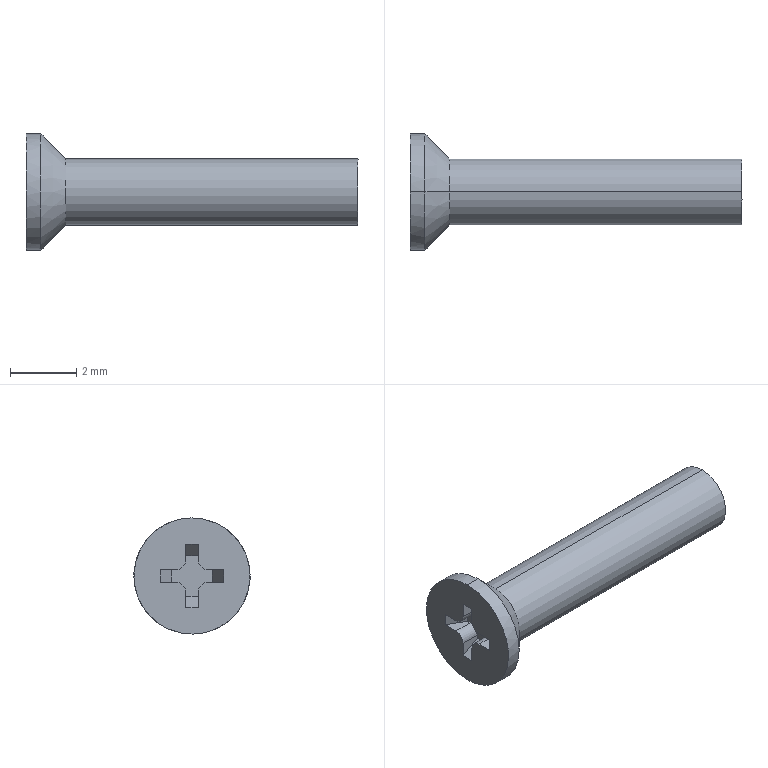Part | STEP file | PN_0016_Default<As Machined> | 1 solid | 25 faces | box 10 x 3.5 x 3.5 mm | volume 35.87 mm3 | plane 15 | cylinder 8 | cone 2 | commonest cylinder face diameters 0.6 x4 2 x2 3.5 x2
STEP:
#1=CARTESIAN_POINT('',(1.2,0.,-1.));
#2=VERTEX_POINT('',#1);
#3=CARTESIAN_POINT('',(1.2,0.,1.));
#4=VERTEX_POINT('',#3);
#5=CARTESIAN_POINT('',(1.2,0.,0.));
#6=DIRECTION('',(1.,0.,0.));
#7=AXIS2_PLACEMENT_3D('',#5,#6,$);
#8=CIRCLE('',#7,1.);
#9=EDGE_CURVE('',#2,#4,#8,.T.);
#10=ORIENTED_EDGE('',*,*,#9,.T.);
#11=CARTESIAN_POINT('',(10.,0.,1.));
#12=VERTEX_POINT('',#11);
#13=CARTESIAN_POINT('',(4.516,0.,1.));
#14=DIRECTION('',(1.,0.,0.));
#15=VECTOR('',#14,1.);
#16=LINE('',#13,#15);
#17=EDGE_CURVE('',#4,#12,#16,.T.);
#18=ORIENTED_EDGE('',*,*,#17,.T.);
#19=CARTESIAN_POINT('',(10.,0.,-1.));
#20=VERTEX_POINT('',#19);
#21=CARTESIAN_POINT('',(10.,0.,0.));
#22=DIRECTION('',(1.,0.,0.));
#23=AXIS2_PLACEMENT_3D('',#21,#22,$);
#24=CIRCLE('',#23,1.);
#25=EDGE_CURVE('',#20,#12,#24,.T.);
#26=ORIENTED_EDGE('',*,*,#25,.F.);
#27=CARTESIAN_POINT('',(4.516,0.,-1.));
#28=DIRECTION('',(1.,0.,0.));
#29=VECTOR('',#28,1.);
#30=LINE('',#27,#29);
#31=EDGE_CURVE('',#2,#20,#30,.T.);
#32=ORIENTED_EDGE('',*,*,#31,.F.);
#33=EDGE_LOOP('',(#10,#18,#26,#32));
#34=FACE_OUTER_BOUND('',#33,.T.);
#35=CARTESIAN_POINT('',(4.516,0.,0.));
#36=DIRECTION('',(1.,0.,0.));
#37=DIRECTION('',(0.,0.,-1.));
#38=AXIS2_PLACEMENT_3D('',#35,#36,#37);
#39=CYLINDRICAL_SURFACE('',#38,1.);
#40=ADVANCED_FACE('',(#34),#39,.T.);
#41=ORIENTED_EDGE('',*,*,#9,.F.);
#42=CARTESIAN_POINT('',(0.45,0.,-1.75));
#43=VERTEX_POINT('',#42);
#44=CARTESIAN_POINT('',(-353551.691,0.,-353553.891));
#45=DIRECTION('',(-0.7071,0.,-0.7071));
#46=VECTOR('',#45,1.);
#47=LINE('',#44,#46);
#48=EDGE_CURVE('',#2,#43,#47,.T.);
#49=ORIENTED_EDGE('',*,*,#48,.T.);
#50=CARTESIAN_POINT('',(0.45,0.,1.75));
#51=VERTEX_POINT('',#50);
#52=CARTESIAN_POINT('',(0.45,0.,0.));
#53=DIRECTION('',(-1.,0.,0.));
#54=AXIS2_PLACEMENT_3D('',#52,#53,$);
#55=CIRCLE('',#54,1.75);
#56=EDGE_CURVE('',#43,#51,#55,.F.);
#57=ORIENTED_EDGE('',*,*,#56,.T.);
#58=CARTESIAN_POINT('',(-353551.691,0.,353553.891));
#59=DIRECTION('',(-0.7071,0.,0.7071));
#60=VECTOR('',#59,1.);
#61=LINE('',#58,#60);
#62=EDGE_CURVE('',#4,#51,#61,.T.);
#63=ORIENTED_EDGE('',*,*,#62,.F.);
#64=EDGE_LOOP('',(#41,#49,#57,#63));
#65=FACE_OUTER_BOUND('',#64,.T.);
#66=CARTESIAN_POINT('',(1.2,0.,0.));
#67=DIRECTION('',(-1.,0.,0.));
#68=DIRECTION('',(0.,0.,1.));
#69=AXIS2_PLACEMENT_3D('',#66,#67,#68);
#70=CONICAL_SURFACE('',#69,1.,0.7854);
#71=ADVANCED_FACE('',(#65),#70,.T.);
#72=ORIENTED_EDGE('',*,*,#17,.F.);
#73=CARTESIAN_POINT('',(1.2,0.,1.));
#74=CARTESIAN_POINT('',(1.2,-0.3142,1.));
#75=CARTESIAN_POINT('',(1.2,-0.6283,0.8766));
#76=CARTESIAN_POINT('',(1.2,-0.8766,0.6283));
#77=CARTESIAN_POINT('',(1.2,-1.123,0.));
#78=CARTESIAN_POINT('',(1.2,-0.8766,-0.6283));
#79=CARTESIAN_POINT('',(1.2,-0.6283,-0.8766));
#80=CARTESIAN_POINT('',(1.2,-0.3142,-1.));
#81=CARTESIAN_POINT('',(1.2,0.,-1.));
#82=B_SPLINE_CURVE_WITH_KNOTS('',5,(#73,#74,#75,#76,#77,#78,#79,#80,#81),.UNSPECIFIED.,.F.,.U.,(6,3,6),(-1.571,0.,1.571),.UNSPECIFIED.);
#83=EDGE_CURVE('',#4,#2,#82,.T.);
#84=ORIENTED_EDGE('',*,*,#83,.T.);
#85=ORIENTED_EDGE('',*,*,#31,.T.);
#86=CARTESIAN_POINT('',(10.,0.,1.));
#87=CARTESIAN_POINT('',(10.,-0.3142,1.));
#88=CARTESIAN_POINT('',(10.,-0.6283,0.8766));
#89=CARTESIAN_POINT('',(10.,-0.8766,0.6283));
#90=CARTESIAN_POINT('',(10.,-1.123,0.));
#91=CARTESIAN_POINT('',(10.,-0.8766,-0.6283));
#92=CARTESIAN_POINT('',(10.,-0.6283,-0.8766));
#93=CARTESIAN_POINT('',(10.,-0.3142,-1.));
#94=CARTESIAN_POINT('',(10.,0.,-1.));
#95=B_SPLINE_CURVE_WITH_KNOTS('',5,(#86,#87,#88,#89,#90,#91,#92,#93,#94),.UNSPECIFIED.,.F.,.U.,(6,3,6),(-1.571,0.,1.571),.UNSPECIFIED.);
#96=EDGE_CURVE('',#12,#20,#95,.T.);
#97=ORIENTED_EDGE('',*,*,#96,.F.);
#98=EDGE_LOOP('',(#72,#84,#85,#97));
#99=FACE_OUTER_BOUND('',#98,.T.);
#100=CARTESIAN_POINT('',(4.516,0.,0.));
#101=DIRECTION('',(1.,0.,0.));
#102=DIRECTION('',(0.,0.,1.));
#103=AXIS2_PLACEMENT_3D('',#100,#101,#102);
#104=CYLINDRICAL_SURFACE('',#103,1.);
#105=ADVANCED_FACE('',(#99),#104,.T.);
#106=ORIENTED_EDGE('',*,*,#25,.T.);
#107=ORIENTED_EDGE('',*,*,#96,.T.);
#108=EDGE_LOOP('',(#106,#107));
#109=FACE_OUTER_BOUND('',#108,.T.);
#110=CARTESIAN_POINT('',(10.,1.,0.));
#111=DIRECTION('',(1.,0.,0.));
#112=DIRECTION('',(0.,0.,-1.));
#113=AXIS2_PLACEMENT_3D('',#110,#111,#112);
#114=PLANE('',#113);
#115=ADVANCED_FACE('',(#109),#114,.T.);
#116=ORIENTED_EDGE('',*,*,#48,.F.);
#117=ORIENTED_EDGE('',*,*,#83,.F.);
#118=ORIENTED_EDGE('',*,*,#62,.T.);
#119=CARTESIAN_POINT('',(0.45,0.,0.));
#120=DIRECTION('',(-1.,0.,0.));
#121=AXIS2_PLACEMENT_3D('',#119,#120,$);
#122=CIRCLE('',#121,1.75);
#123=EDGE_CURVE('',#51,#43,#122,.F.);
#124=ORIENTED_EDGE('',*,*,#123,.T.);
#125=EDGE_LOOP('',(#116,#117,#118,#124));
#126=FACE_OUTER_BOUND('',#125,.T.);
#127=CARTESIAN_POINT('',(1.2,0.,0.));
#128=DIRECTION('',(-1.,0.,0.));
#129=DIRECTION('',(0.,0.,-1.));
#130=AXIS2_PLACEMENT_3D('',#127,#128,#129);
#131=CONICAL_SURFACE('',#130,1.,0.7854);
#132=ADVANCED_FACE('',(#126),#131,.T.);
#133=CARTESIAN_POINT('',(0.,0.,-1.75));
#134=VERTEX_POINT('',#133);
#135=CARTESIAN_POINT('',(0.,0.,1.75));
#136=VERTEX_POINT('',#135);
#137=CARTESIAN_POINT('',(0.,0.,-1.75));
#138=CARTESIAN_POINT('',(0.,0.5498,-1.75));
#139=CARTESIAN_POINT('',(0.,1.1,-1.534));
#140=CARTESIAN_POINT('',(0.,1.534,-1.1));
#141=CARTESIAN_POINT('',(0.,1.966,0.));
#142=CARTESIAN_POINT('',(0.,1.534,1.1));
#143=CARTESIAN_POINT('',(0.,1.1,1.534));
#144=CARTESIAN_POINT('',(0.,0.5498,1.75));
#145=CARTESIAN_POINT('',(0.,0.,1.75));
#146=B_SPLINE_CURVE_WITH_KNOTS('',5,(#137,#138,#139,#140,#141,#142,#143,#144,#145),.UNSPECIFIED.,.F.,.U.,(6,3,6),(-2.749,0.,2.749),.UNSPECIFIED.);
#147=EDGE_CURVE('',#134,#136,#146,.T.);
#148=ORIENTED_EDGE('',*,*,#147,.T.);
#149=CARTESIAN_POINT('',(4.516,0.,1.75));
#150=DIRECTION('',(1.,0.,0.));
#151=VECTOR('',#150,1.);
#152=LINE('',#149,#151);
#153=EDGE_CURVE('',#136,#51,#152,.T.);
#154=ORIENTED_EDGE('',*,*,#153,.T.);
#155=ORIENTED_EDGE('',*,*,#56,.F.);
#156=CARTESIAN_POINT('',(4.516,0.,-1.75));
#157=DIRECTION('',(1.,0.,0.));
#158=VECTOR('',#157,1.);
#159=LINE('',#156,#158);
#160=EDGE_CURVE('',#134,#43,#159,.T.);
#161=ORIENTED_EDGE('',*,*,#160,.F.);
#162=EDGE_LOOP('',(#148,#154,#155,#161));
#163=FACE_OUTER_BOUND('',#162,.T.);
#164=CARTESIAN_POINT('',(4.516,0.,0.));
#165=DIRECTION('',(1.,0.,0.));
#166=DIRECTION('',(0.,0.,-1.));
#167=AXIS2_PLACEMENT_3D('',#164,#165,#166);
#168=CYLINDRICAL_SURFACE('',#167,1.75);
#169=ADVANCED_FACE('',(#163),#168,.T.);
#170=ORIENTED_EDGE('',*,*,#153,.F.);
#171=CARTESIAN_POINT('',(0.,0.,1.75));
#172=CARTESIAN_POINT('',(0.,-0.5498,1.75));
#173=CARTESIAN_POINT('',(0.,-1.1,1.534));
#174=CARTESIAN_POINT('',(0.,-1.534,1.1));
#175=CARTESIAN_POINT('',(0.,-1.966,0.));
#176=CARTESIAN_POINT('',(0.,-1.534,-1.1));
#177=CARTESIAN_POINT('',(0.,-1.1,-1.534));
#178=CARTESIAN_POINT('',(0.,-0.5498,-1.75));
#179=CARTESIAN_POINT('',(0.,0.,-1.75));
#180=B_SPLINE_CURVE_WITH_KNOTS('',5,(#171,#172,#173,#174,#175,#176,#177,#178,#179),.UNSPECIFIED.,.F.,.U.,(6,3,6),(-2.749,0.,2.749),.UNSPECIFIED.);
#181=EDGE_CURVE('',#136,#134,#180,.T.);
#182=ORIENTED_EDGE('',*,*,#181,.T.);
#183=ORIENTED_EDGE('',*,*,#160,.T.);
#184=ORIENTED_EDGE('',*,*,#123,.F.);
#185=EDGE_LOOP('',(#170,#182,#183,#184));
#186=FACE_OUTER_BOUND('',#185,.T.);
#187=CARTESIAN_POINT('',(4.516,0.,0.));
#188=DIRECTION('',(1.,0.,0.));
#189=DIRECTION('',(0.,0.,1.));
#190=AXIS2_PLACEMENT_3D('',#187,#188,#189);
#191=CYLINDRICAL_SURFACE('',#190,1.75);
#192=ADVANCED_FACE('',(#186),#191,.T.);
#193=ORIENTED_EDGE('',*,*,#147,.F.);
#194=ORIENTED_EDGE('',*,*,#181,.F.);
#195=EDGE_LOOP('',(#193,#194));
#196=FACE_OUTER_BOUND('',#195,.T.);
#197=CARTESIAN_POINT('',(0.,-0.95,-0.19));
#198=VERTEX_POINT('',#197);
#199=CARTESIAN_POINT('',(0.,-0.49,-0.19));
#200=VERTEX_POINT('',#199);
#201=CARTESIAN_POINT('',(0.,-0.72,-0.19));
#202=DIRECTION('',(0.,1.,0.));
#203=VECTOR('',#202,1.);
#204=LINE('',#201,#203);
#205=EDGE_CURVE('',#198,#200,#204,.T.);
#206=ORIENTED_EDGE('',*,*,#205,.T.);
#207=CARTESIAN_POINT('',(0.,-0.19,-0.49));
#208=VERTEX_POINT('',#207);
#209=CARTESIAN_POINT('',(0.,-0.49,-0.49));
#210=DIRECTION('',(-1.,0.,0.));
#211=AXIS2_PLACEMENT_3D('',#209,#210,$);
#212=CIRCLE('',#211,0.3);
#213=EDGE_CURVE('',#200,#208,#212,.T.);
#214=ORIENTED_EDGE('',*,*,#213,.T.);
#215=CARTESIAN_POINT('',(0.,-0.19,-0.95));
#216=VERTEX_POINT('',#215);
#217=CARTESIAN_POINT('',(0.,-0.19,-0.72));
#218=DIRECTION('',(0.,0.,-1.));
#219=VECTOR('',#218,1.);
#220=LINE('',#217,#219);
#221=EDGE_CURVE('',#208,#216,#220,.T.);
#222=ORIENTED_EDGE('',*,*,#221,.T.);
#223=CARTESIAN_POINT('',(0.,0.19,-0.95));
#224=VERTEX_POINT('',#223);
#225=CARTESIAN_POINT('',(0.,0.,-0.95));
#226=DIRECTION('',(0.,1.,0.));
#227=VECTOR('',#226,1.);
#228=LINE('',#225,#227);
#229=EDGE_CURVE('',#216,#224,#228,.T.);
#230=ORIENTED_EDGE('',*,*,#229,.T.);
#231=CARTESIAN_POINT('',(0.,0.19,-0.49));
#232=VERTEX_POINT('',#231);
#233=CARTESIAN_POINT('',(0.,0.19,-0.72));
#234=DIRECTION('',(0.,0.,1.));
#235=VECTOR('',#234,1.);
#236=LINE('',#233,#235);
#237=EDGE_CURVE('',#224,#232,#236,.T.);
#238=ORIENTED_EDGE('',*,*,#237,.T.);
#239=CARTESIAN_POINT('',(0.,0.49,-0.19));
#240=VERTEX_POINT('',#239);
#241=CARTESIAN_POINT('',(0.,0.49,-0.49));
#242=DIRECTION('',(-1.,0.,0.));
#243=AXIS2_PLACEMENT_3D('',#241,#242,$);
#244=CIRCLE('',#243,0.3);
#245=EDGE_CURVE('',#232,#240,#244,.T.);
#246=ORIENTED_EDGE('',*,*,#245,.T.);
#247=CARTESIAN_POINT('',(0.,0.95,-0.19));
#248=VERTEX_POINT('',#247);
#249=CARTESIAN_POINT('',(0.,0.72,-0.19));
#250=DIRECTION('',(0.,1.,0.));
#251=VECTOR('',#250,1.);
#252=LINE('',#249,#251);
#253=EDGE_CURVE('',#240,#248,#252,.T.);
#254=ORIENTED_EDGE('',*,*,#253,.T.);
#255=CARTESIAN_POINT('',(0.,0.95,0.19));
#256=VERTEX_POINT('',#255);
#257=CARTESIAN_POINT('',(0.,0.95,0.));
#258=DIRECTION('',(0.,0.,1.));
#259=VECTOR('',#258,1.);
#260=LINE('',#257,#259);
#261=EDGE_CURVE('',#248,#256,#260,.T.);
#262=ORIENTED_EDGE('',*,*,#261,.T.);
#263=CARTESIAN_POINT('',(0.,0.49,0.19));
#264=VERTEX_POINT('',#263);
#265=CARTESIAN_POINT('',(0.,0.72,0.19));
#266=DIRECTION('',(0.,-1.,0.));
#267=VECTOR('',#266,1.);
#268=LINE('',#265,#267);
#269=EDGE_CURVE('',#256,#264,#268,.T.);
#270=ORIENTED_EDGE('',*,*,#269,.T.);
#271=CARTESIAN_POINT('',(0.,0.19,0.49));
#272=VERTEX_POINT('',#271);
#273=CARTESIAN_POINT('',(0.,0.49,0.49));
#274=DIRECTION('',(-1.,0.,0.));
#275=AXIS2_PLACEMENT_3D('',#273,#274,$);
#276=CIRCLE('',#275,0.3);
#277=EDGE_CURVE('',#264,#272,#276,.T.);
#278=ORIENTED_EDGE('',*,*,#277,.T.);
#279=CARTESIAN_POINT('',(0.,0.19,0.95));
#280=VERTEX_POINT('',#279);
#281=CARTESIAN_POINT('',(0.,0.19,0.72));
#282=DIRECTION('',(0.,0.,1.));
#283=VECTOR('',#282,1.);
#284=LINE('',#281,#283);
#285=EDGE_CURVE('',#272,#280,#284,.T.);
#286=ORIENTED_EDGE('',*,*,#285,.T.);
#287=CARTESIAN_POINT('',(0.,-0.19,0.95));
#288=VERTEX_POINT('',#287);
#289=CARTESIAN_POINT('',(0.,0.,0.95));
#290=DIRECTION('',(0.,-1.,0.));
#291=VECTOR('',#290,1.);
#292=LINE('',#289,#291);
#293=EDGE_CURVE('',#280,#288,#292,.T.);
#294=ORIENTED_EDGE('',*,*,#293,.T.);
#295=CARTESIAN_POINT('',(0.,-0.19,0.49));
#296=VERTEX_POINT('',#295);
#297=CARTESIAN_POINT('',(0.,-0.19,0.72));
#298=DIRECTION('',(0.,0.,-1.));
#299=VECTOR('',#298,1.);
#300=LINE('',#297,#299);
#301=EDGE_CURVE('',#288,#296,#300,.T.);
#302=ORIENTED_EDGE('',*,*,#301,.T.);
#303=CARTESIAN_POINT('',(0.,-0.49,0.19));
#304=VERTEX_POINT('',#303);
#305=CARTESIAN_POINT('',(0.,-0.49,0.49));
#306=DIRECTION('',(-1.,0.,0.));
#307=AXIS2_PLACEMENT_3D('',#305,#306,$);
#308=CIRCLE('',#307,0.3);
#309=EDGE_CURVE('',#296,#304,#308,.T.);
#310=ORIENTED_EDGE('',*,*,#309,.T.);
#311=CARTESIAN_POINT('',(0.,-0.95,0.19));
#312=VERTEX_POINT('',#311);
#313=CARTESIAN_POINT('',(0.,-0.72,0.19));
#314=DIRECTION('',(0.,-1.,0.));
#315=VECTOR('',#314,1.);
#316=LINE('',#313,#315);
#317=EDGE_CURVE('',#304,#312,#316,.T.);
#318=ORIENTED_EDGE('',*,*,#317,.T.);
#319=CARTESIAN_POINT('',(0.,-0.95,0.));
#320=DIRECTION('',(0.,0.,-1.));
#321=VECTOR('',#320,1.);
#322=LINE('',#319,#321);
#323=EDGE_CURVE('',#312,#198,#322,.T.);
#324=ORIENTED_EDGE('',*,*,#323,.T.);
#325=EDGE_LOOP('',(#206,#214,#222,#230,#238,#246,#254,#262,#270,#278,#286,#294,#302,#310,#318,#324));
#326=FACE_BOUND('',#325,.T.);
#327=CARTESIAN_POINT('',(0.,1.75,0.));
#328=DIRECTION('',(-1.,0.,0.));
#329=DIRECTION('',(0.,0.,1.));
#330=AXIS2_PLACEMENT_3D('',#327,#328,#329);
#331=PLANE('',#330);
#332=ADVANCED_FACE('',(#196,#326),#331,.T.);
#333=CARTESIAN_POINT('',(0.6,-0.6036,-0.19));
#334=VERTEX_POINT('',#333);
#335=CARTESIAN_POINT('',(0.6,-0.49,-0.19));
#336=VERTEX_POINT('',#335);
#337=CARTESIAN_POINT('',(0.6,-0.5468,-0.19));
#338=DIRECTION('',(0.,1.,0.));
#339=VECTOR('',#338,1.);
#340=LINE('',#337,#339);
#341=EDGE_CURVE('',#334,#336,#340,.T.);
#342=ORIENTED_EDGE('',*,*,#341,.T.);
#343=CARTESIAN_POINT('',(0.3,-0.49,-0.19));
#344=DIRECTION('',(-1.,0.,0.));
#345=VECTOR('',#344,1.);
#346=LINE('',#343,#345);
#347=EDGE_CURVE('',#336,#200,#346,.T.);
#348=ORIENTED_EDGE('',*,*,#347,.T.);
#349=ORIENTED_EDGE('',*,*,#205,.F.);
#350=CARTESIAN_POINT('',(0.3,-0.7768,-0.19));
#351=DIRECTION('',(-0.866,-0.5,0.));
#352=VECTOR('',#351,1.);
#353=LINE('',#350,#352);
#354=EDGE_CURVE('',#334,#198,#353,.T.);
#355=ORIENTED_EDGE('',*,*,#354,.F.);
#356=EDGE_LOOP('',(#342,#348,#349,#355));
#357=FACE_OUTER_BOUND('',#356,.T.);
#358=CARTESIAN_POINT('',(0.6,-0.19,-0.19));
#359=DIRECTION('',(0.,0.,1.));
#360=DIRECTION('',(1.,0.,0.));
#361=AXIS2_PLACEMENT_3D('',#358,#359,#360);
#362=PLANE('',#361);
#363=ADVANCED_FACE('',(#357),#362,.T.);
#364=CARTESIAN_POINT('',(0.6,-0.19,-0.49));
#365=VERTEX_POINT('',#364);
#366=CARTESIAN_POINT('',(0.6,-0.49,-0.49));
#367=DIRECTION('',(-1.,0.,0.));
#368=AXIS2_PLACEMENT_3D('',#366,#367,$);
#369=CIRCLE('',#368,0.3);
#370=EDGE_CURVE('',#365,#336,#369,.F.);
#371=ORIENTED_EDGE('',*,*,#370,.F.);
#372=CARTESIAN_POINT('',(0.6,-0.19,-0.49));
#373=DIRECTION('',(-1.,0.,0.));
#374=VECTOR('',#373,1.);
#375=LINE('',#372,#374);
#376=EDGE_CURVE('',#208,#365,#375,.F.);
#377=ORIENTED_EDGE('',*,*,#376,.F.);
#378=ORIENTED_EDGE('',*,*,#213,.F.);
#379=ORIENTED_EDGE('',*,*,#347,.F.);
#380=EDGE_LOOP('',(#371,#377,#378,#379));
#381=FACE_OUTER_BOUND('',#380,.T.);
#382=CARTESIAN_POINT('',(0.6,-0.49,-0.49));
#383=DIRECTION('',(-1.,0.,0.));
#384=DIRECTION('',(0.,0.,1.));
#385=AXIS2_PLACEMENT_3D('',#382,#383,#384);
#386=CYLINDRICAL_SURFACE('',#385,0.3);
#387=ADVANCED_FACE('',(#381),#386,.T.);
#388=ORIENTED_EDGE('',*,*,#221,.F.);
#389=ORIENTED_EDGE('',*,*,#376,.T.);
#390=CARTESIAN_POINT('',(0.6,-0.19,-0.6036));
#391=VERTEX_POINT('',#390);
#392=CARTESIAN_POINT('',(0.6,-0.19,-0.5468));
#393=DIRECTION('',(0.,0.,-1.));
#394=VECTOR('',#393,1.);
#395=LINE('',#392,#394);
#396=EDGE_CURVE('',#365,#391,#395,.T.);
#397=ORIENTED_EDGE('',*,*,#396,.T.);
#398=CARTESIAN_POINT('',(0.3,-0.19,-0.7768));
#399=DIRECTION('',(-0.866,0.,-0.5));
#400=VECTOR('',#399,1.);
#401=LINE('',#398,#400);
#402=EDGE_CURVE('',#391,#216,#401,.T.);
#403=ORIENTED_EDGE('',*,*,#402,.T.);
#404=EDGE_LOOP('',(#388,#389,#397,#403));
#405=FACE_OUTER_BOUND('',#404,.T.);
#406=CARTESIAN_POINT('',(0.6,-0.19,-0.19));
#407=DIRECTION('',(0.,1.,0.));
#408=DIRECTION('',(0.,0.,1.));
#409=AXIS2_PLACEMENT_3D('',#406,#407,#408);
#410=PLANE('',#409);
#411=ADVANCED_FACE('',(#405),#410,.T.);
#412=ORIENTED_EDGE('',*,*,#229,.F.);
#413=ORIENTED_EDGE('',*,*,#402,.F.);
#414=CARTESIAN_POINT('',(0.6,0.19,-0.6036));
#415=VERTEX_POINT('',#414);
#416=CARTESIAN_POINT('',(0.6,0.,-0.6036));
#417=DIRECTION('',(0.,1.,0.));
#418=VECTOR('',#417,1.);
#419=LINE('',#416,#418);
#420=EDGE_CURVE('',#391,#415,#419,.T.);
#421=ORIENTED_EDGE('',*,*,#420,.T.);
#422=CARTESIAN_POINT('',(0.3,0.19,-0.7768));
#423=DIRECTION('',(-0.866,0.,-0.5));
#424=VECTOR('',#423,1.);
#425=LINE('',#422,#424);
#426=EDGE_CURVE('',#415,#224,#425,.T.);
#427=ORIENTED_EDGE('',*,*,#426,.T.);
#428=EDGE_LOOP('',(#412,#413,#421,#427));
#429=FACE_OUTER_BOUND('',#428,.T.);
#430=CARTESIAN_POINT('',(0.,0.19,-0.95));
#431=DIRECTION('',(-0.5,0.,0.866));
#432=DIRECTION('',(0.866,0.,0.5));
#433=AXIS2_PLACEMENT_3D('',#430,#431,#432);
#434=PLANE('',#433);
#435=ADVANCED_FACE('',(#429),#434,.T.);
#436=CARTESIAN_POINT('',(0.6,0.19,-0.49));
#437=VERTEX_POINT('',#436);
#438=CARTESIAN_POINT('',(0.6,0.19,-0.5468));
#439=DIRECTION('',(0.,0.,1.));
#440=VECTOR('',#439,1.);
#441=LINE('',#438,#440);
#442=EDGE_CURVE('',#415,#437,#441,.T.);
#443=ORIENTED_EDGE('',*,*,#442,.T.);
#444=CARTESIAN_POINT('',(0.3,0.19,-0.49));
#445=DIRECTION('',(-1.,0.,0.));
#446=VECTOR('',#445,1.);
#447=LINE('',#444,#446);
#448=EDGE_CURVE('',#437,#232,#447,.T.);
#449=ORIENTED_EDGE('',*,*,#448,.T.);
#450=ORIENTED_EDGE('',*,*,#237,.F.);
#451=ORIENTED_EDGE('',*,*,#426,.F.);
#452=EDGE_LOOP('',(#443,#449,#450,#451));
#453=FACE_OUTER_BOUND('',#452,.T.);
#454=CARTESIAN_POINT('',(0.6,0.19,-0.19));
#455=DIRECTION('',(0.,-1.,0.));
#456=DIRECTION('',(0.,0.,-1.));
#457=AXIS2_PLACEMENT_3D('',#454,#455,#456);
#458=PLANE('',#457);
#459=ADVANCED_FACE('',(#453),#458,.T.);
#460=CARTESIAN_POINT('',(0.6,0.49,-0.19));
#461=VERTEX_POINT('',#460);
#462=CARTESIAN_POINT('',(0.6,0.49,-0.49));
#463=DIRECTION('',(-1.,0.,0.));
#464=AXIS2_PLACEMENT_3D('',#462,#463,$);
#465=CIRCLE('',#464,0.3);
#466=EDGE_CURVE('',#461,#437,#465,.F.);
#467=ORIENTED_EDGE('',*,*,#466,.F.);
#468=CARTESIAN_POINT('',(0.6,0.49,-0.19));
#469=DIRECTION('',(-1.,0.,0.));
#470=VECTOR('',#469,1.);
#471=LINE('',#468,#470);
#472=EDGE_CURVE('',#240,#461,#471,.F.);
#473=ORIENTED_EDGE('',*,*,#472,.F.);
#474=ORIENTED_EDGE('',*,*,#245,.F.);
#475=ORIENTED_EDGE('',*,*,#448,.F.);
#476=EDGE_LOOP('',(#467,#473,#474,#475));
#477=FACE_OUTER_BOUND('',#476,.T.);
#478=CARTESIAN_POINT('',(0.6,0.49,-0.49));
#479=DIRECTION('',(-1.,0.,0.));
#480=DIRECTION('',(0.,0.,-1.));
#481=AXIS2_PLACEMENT_3D('',#478,#479,#480);
#482=CYLINDRICAL_SURFACE('',#481,0.3);
#483=ADVANCED_FACE('',(#477),#482,.T.);
#484=ORIENTED_EDGE('',*,*,#253,.F.);
#485=ORIENTED_EDGE('',*,*,#472,.T.);
#486=CARTESIAN_POINT('',(0.6,0.6036,-0.19));
#487=VERTEX_POINT('',#486);
#488=CARTESIAN_POINT('',(0.6,0.5468,-0.19));
#489=DIRECTION('',(0.,1.,0.));
#490=VECTOR('',#489,1.);
#491=LINE('',#488,#490);
#492=EDGE_CURVE('',#461,#487,#491,.T.);
#493=ORIENTED_EDGE('',*,*,#492,.T.);
#494=CARTESIAN_POINT('',(0.3,0.7768,-0.19));
#495=DIRECTION('',(-0.866,0.5,0.));
#496=VECTOR('',#495,1.);
#497=LINE('',#494,#496);
#498=EDGE_CURVE('',#487,#248,#497,.T.);
#499=ORIENTED_EDGE('',*,*,#498,.T.);
#500=EDGE_LOOP('',(#484,#485,#493,#499));
#501=FACE_OUTER_BOUND('',#500,.T.);
#502=CARTESIAN_POINT('',(0.6,0.19,-0.19));
#503=DIRECTION('',(0.,0.,1.));
#504=DIRECTION('',(1.,0.,0.));
#505=AXIS2_PLACEMENT_3D('',#502,#503,#504);
#506=PLANE('',#505);
#507=ADVANCED_FACE('',(#501),#506,.T.);
#508=ORIENTED_EDGE('',*,*,#261,.F.);
#509=ORIENTED_EDGE('',*,*,#498,.F.);
#510=CARTESIAN_POINT('',(0.6,0.6036,0.19));
#511=VERTEX_POINT('',#510);
#512=CARTESIAN_POINT('',(0.6,0.6036,0.));
#513=DIRECTION('',(0.,0.,1.));
#514=VECTOR('',#513,1.);
#515=LINE('',#512,#514);
#516=EDGE_CURVE('',#487,#511,#515,.T.);
#517=ORIENTED_EDGE('',*,*,#516,.T.);
#518=CARTESIAN_POINT('',(0.3,0.7768,0.19));
#519=DIRECTION('',(-0.866,0.5,0.));
#520=VECTOR('',#519,1.);
#521=LINE('',#518,#520);
#522=EDGE_CURVE('',#511,#256,#521,.T.);
#523=ORIENTED_EDGE('',*,*,#522,.T.);
#524=EDGE_LOOP('',(#508,#509,#517,#523));
#525=FACE_OUTER_BOUND('',#524,.T.);
#526=CARTESIAN_POINT('',(0.,0.95,-0.19));
#527=DIRECTION('',(-0.5,-0.866,0.));
#528=DIRECTION('',(0.866,-0.5,0.));
#529=AXIS2_PLACEMENT_3D('',#526,#527,#528);
#530=PLANE('',#529);
#531=ADVANCED_FACE('',(#525),#530,.T.);
#532=CARTESIAN_POINT('',(0.6,0.49,0.19));
#533=VERTEX_POINT('',#532);
#534=CARTESIAN_POINT('',(0.6,0.5468,0.19));
#535=DIRECTION('',(0.,-1.,0.));
#536=VECTOR('',#535,1.);
#537=LINE('',#534,#536);
#538=EDGE_CURVE('',#511,#533,#537,.T.);
#539=ORIENTED_EDGE('',*,*,#538,.T.);
#540=CARTESIAN_POINT('',(0.3,0.49,0.19));
#541=DIRECTION('',(-1.,0.,0.));
#542=VECTOR('',#541,1.);
#543=LINE('',#540,#542);
#544=EDGE_CURVE('',#533,#264,#543,.T.);
#545=ORIENTED_EDGE('',*,*,#544,.T.);
#546=ORIENTED_EDGE('',*,*,#269,.F.);
#547=ORIENTED_EDGE('',*,*,#522,.F.);
#548=EDGE_LOOP('',(#539,#545,#546,#547));
#549=FACE_OUTER_BOUND('',#548,.T.);
#550=CARTESIAN_POINT('',(0.6,0.19,0.19));
#551=DIRECTION('',(0.,0.,-1.));
#552=DIRECTION('',(0.,1.,0.));
#553=AXIS2_PLACEMENT_3D('',#550,#551,#552);
#554=PLANE('',#553);
#555=ADVANCED_FACE('',(#549),#554,.T.);
#556=CARTESIAN_POINT('',(0.6,0.19,0.49));
#557=VERTEX_POINT('',#556);
#558=CARTESIAN_POINT('',(0.6,0.49,0.49));
#559=DIRECTION('',(-1.,0.,0.));
#560=AXIS2_PLACEMENT_3D('',#558,#559,$);
#561=CIRCLE('',#560,0.3);
#562=EDGE_CURVE('',#557,#533,#561,.F.);
#563=ORIENTED_EDGE('',*,*,#562,.F.);
#564=CARTESIAN_POINT('',(0.6,0.19,0.49));
#565=DIRECTION('',(-1.,0.,0.));
#566=VECTOR('',#565,1.);
#567=LINE('',#564,#566);
#568=EDGE_CURVE('',#272,#557,#567,.F.);
#569=ORIENTED_EDGE('',*,*,#568,.F.);
#570=ORIENTED_EDGE('',*,*,#277,.F.);
#571=ORIENTED_EDGE('',*,*,#544,.F.);
#572=EDGE_LOOP('',(#563,#569,#570,#571));
#573=FACE_OUTER_BOUND('',#572,.T.);
#574=CARTESIAN_POINT('',(0.6,0.49,0.49));
#575=DIRECTION('',(-1.,0.,0.));
#576=DIRECTION('',(0.,0.,-1.));
#577=AXIS2_PLACEMENT_3D('',#574,#575,#576);
#578=CYLINDRICAL_SURFACE('',#577,0.3);
#579=ADVANCED_FACE('',(#573),#578,.T.);
#580=ORIENTED_EDGE('',*,*,#285,.F.);
#581=ORIENTED_EDGE('',*,*,#568,.T.);
#582=CARTESIAN_POINT('',(0.6,0.19,0.6036));
#583=VERTEX_POINT('',#582);
#584=CARTESIAN_POINT('',(0.6,0.19,0.5468));
#585=DIRECTION('',(0.,0.,1.));
#586=VECTOR('',#585,1.);
#587=LINE('',#584,#586);
#588=EDGE_CURVE('',#557,#583,#587,.T.);
#589=ORIENTED_EDGE('',*,*,#588,.T.);
#590=CARTESIAN_POINT('',(0.3,0.19,0.7768));
#591=DIRECTION('',(-0.866,0.,0.5));
#592=VECTOR('',#591,1.);
#593=LINE('',#590,#592);
#594=EDGE_CURVE('',#583,#280,#593,.T.);
#595=ORIENTED_EDGE('',*,*,#594,.T.);
#596=EDGE_LOOP('',(#580,#581,#589,#595));
#597=FACE_OUTER_BOUND('',#596,.T.);
#598=CARTESIAN_POINT('',(0.6,0.19,0.19));
#599=DIRECTION('',(0.,-1.,0.));
#600=DIRECTION('',(0.,0.,-1.));
#601=AXIS2_PLACEMENT_3D('',#598,#599,#600);
#602=PLANE('',#601);
#603=ADVANCED_FACE('',(#597),#602,.T.);
#604=ORIENTED_EDGE('',*,*,#293,.F.);
#605=ORIENTED_EDGE('',*,*,#594,.F.);
#606=CARTESIAN_POINT('',(0.6,-0.19,0.6036));
#607=VERTEX_POINT('',#606);
#608=CARTESIAN_POINT('',(0.6,0.,0.6036));
#609=DIRECTION('',(0.,-1.,0.));
#610=VECTOR('',#609,1.);
#611=LINE('',#608,#610);
#612=EDGE_CURVE('',#583,#607,#611,.T.);
#613=ORIENTED_EDGE('',*,*,#612,.T.);
#614=CARTESIAN_POINT('',(0.3,-0.19,0.7768));
#615=DIRECTION('',(-0.866,0.,0.5));
#616=VECTOR('',#615,1.);
#617=LINE('',#614,#616);
#618=EDGE_CURVE('',#607,#288,#617,.T.);
#619=ORIENTED_EDGE('',*,*,#618,.T.);
#620=EDGE_LOOP('',(#604,#605,#613,#619));
#621=FACE_OUTER_BOUND('',#620,.T.);
#622=CARTESIAN_POINT('',(0.,0.19,0.95));
#623=DIRECTION('',(-0.5,0.,-0.866));
#624=DIRECTION('',(-0.866,0.,0.5));
#625=AXIS2_PLACEMENT_3D('',#622,#623,#624);
#626=PLANE('',#625);
#627=ADVANCED_FACE('',(#621),#626,.T.);
#628=CARTESIAN_POINT('',(0.6,-0.19,0.49));
#629=VERTEX_POINT('',#628);
#630=CARTESIAN_POINT('',(0.6,-0.19,0.5468));
#631=DIRECTION('',(0.,0.,-1.));
#632=VECTOR('',#631,1.);
#633=LINE('',#630,#632);
#634=EDGE_CURVE('',#607,#629,#633,.T.);
#635=ORIENTED_EDGE('',*,*,#634,.T.);
#636=CARTESIAN_POINT('',(0.3,-0.19,0.49));
#637=DIRECTION('',(-1.,0.,0.));
#638=VECTOR('',#637,1.);
#639=LINE('',#636,#638);
#640=EDGE_CURVE('',#629,#296,#639,.T.);
#641=ORIENTED_EDGE('',*,*,#640,.T.);
#642=ORIENTED_EDGE('',*,*,#301,.F.);
#643=ORIENTED_EDGE('',*,*,#618,.F.);
#644=EDGE_LOOP('',(#635,#641,#642,#643));
#645=FACE_OUTER_BOUND('',#644,.T.);
#646=CARTESIAN_POINT('',(0.6,-0.19,0.19));
#647=DIRECTION('',(0.,1.,0.));
#648=DIRECTION('',(0.,0.,1.));
#649=AXIS2_PLACEMENT_3D('',#646,#647,#648);
#650=PLANE('',#649);
#651=ADVANCED_FACE('',(#645),#650,.T.);
#652=CARTESIAN_POINT('',(0.6,-0.49,0.19));
#653=VERTEX_POINT('',#652);
#654=CARTESIAN_POINT('',(0.6,-0.49,0.49));
#655=DIRECTION('',(-1.,0.,0.));
#656=AXIS2_PLACEMENT_3D('',#654,#655,$);
#657=CIRCLE('',#656,0.3);
#658=EDGE_CURVE('',#653,#629,#657,.F.);
#659=ORIENTED_EDGE('',*,*,#658,.F.);
#660=CARTESIAN_POINT('',(0.6,-0.49,0.19));
#661=DIRECTION('',(-1.,0.,0.));
#662=VECTOR('',#661,1.);
#663=LINE('',#660,#662);
#664=EDGE_CURVE('',#304,#653,#663,.F.);
#665=ORIENTED_EDGE('',*,*,#664,.F.);
#666=ORIENTED_EDGE('',*,*,#309,.F.);
#667=ORIENTED_EDGE('',*,*,#640,.F.);
#668=EDGE_LOOP('',(#659,#665,#666,#667));
#669=FACE_OUTER_BOUND('',#668,.T.);
#670=CARTESIAN_POINT('',(0.6,-0.49,0.49));
#671=DIRECTION('',(-1.,0.,0.));
#672=DIRECTION('',(0.,0.,1.));
#673=AXIS2_PLACEMENT_3D('',#670,#671,#672);
#674=CYLINDRICAL_SURFACE('',#673,0.3);
#675=ADVANCED_FACE('',(#669),#674,.T.);
#676=ORIENTED_EDGE('',*,*,#317,.F.);
#677=ORIENTED_EDGE('',*,*,#664,.T.);
#678=CARTESIAN_POINT('',(0.6,-0.6036,0.19));
#679=VERTEX_POINT('',#678);
#680=CARTESIAN_POINT('',(0.6,-0.5468,0.19));
#681=DIRECTION('',(0.,-1.,0.));
#682=VECTOR('',#681,1.);
#683=LINE('',#680,#682);
#684=EDGE_CURVE('',#653,#679,#683,.T.);
#685=ORIENTED_EDGE('',*,*,#684,.T.);
#686=CARTESIAN_POINT('',(0.3,-0.7768,0.19));
#687=DIRECTION('',(-0.866,-0.5,0.));
#688=VECTOR('',#687,1.);
#689=LINE('',#686,#688);
#690=EDGE_CURVE('',#679,#312,#689,.T.);
#691=ORIENTED_EDGE('',*,*,#690,.T.);
#692=EDGE_LOOP('',(#676,#677,#685,#691));
#693=FACE_OUTER_BOUND('',#692,.T.);
#694=CARTESIAN_POINT('',(0.6,-0.19,0.19));
#695=DIRECTION('',(0.,0.,-1.));
#696=DIRECTION('',(0.,1.,0.));
#697=AXIS2_PLACEMENT_3D('',#694,#695,#696);
#698=PLANE('',#697);
#699=ADVANCED_FACE('',(#693),#698,.T.);
#700=ORIENTED_EDGE('',*,*,#323,.F.);
#701=ORIENTED_EDGE('',*,*,#690,.F.);
#702=CARTESIAN_POINT('',(0.6,-0.6036,0.));
#703=DIRECTION('',(0.,0.,-1.));
#704=VECTOR('',#703,1.);
#705=LINE('',#702,#704);
#706=EDGE_CURVE('',#679,#334,#705,.T.);
#707=ORIENTED_EDGE('',*,*,#706,.T.);
#708=ORIENTED_EDGE('',*,*,#354,.T.);
#709=EDGE_LOOP('',(#700,#701,#707,#708));
#710=FACE_OUTER_BOUND('',#709,.T.);
#711=CARTESIAN_POINT('',(0.,-0.95,-0.19));
#712=DIRECTION('',(-0.5,0.866,0.));
#713=DIRECTION('',(-0.866,-0.5,0.));
#714=AXIS2_PLACEMENT_3D('',#711,#712,#713);
#715=PLANE('',#714);
#716=ADVANCED_FACE('',(#710),#715,.T.);
#717=ORIENTED_EDGE('',*,*,#588,.F.);
#718=ORIENTED_EDGE('',*,*,#562,.T.);
#719=ORIENTED_EDGE('',*,*,#538,.F.);
#720=ORIENTED_EDGE('',*,*,#516,.F.);
#721=ORIENTED_EDGE('',*,*,#492,.F.);
#722=ORIENTED_EDGE('',*,*,#466,.T.);
#723=ORIENTED_EDGE('',*,*,#442,.F.);
#724=ORIENTED_EDGE('',*,*,#420,.F.);
#725=ORIENTED_EDGE('',*,*,#396,.F.);
#726=ORIENTED_EDGE('',*,*,#370,.T.);
#727=ORIENTED_EDGE('',*,*,#341,.F.);
#728=ORIENTED_EDGE('',*,*,#706,.F.);
#729=ORIENTED_EDGE('',*,*,#684,.F.);
#730=ORIENTED_EDGE('',*,*,#658,.T.);
#731=ORIENTED_EDGE('',*,*,#634,.F.);
#732=ORIENTED_EDGE('',*,*,#612,.F.);
#733=EDGE_LOOP('',(#717,#718,#719,#720,#721,#722,#723,#724,#725,#726,#727,#728,#729,#730,#731,#732));
#734=FACE_OUTER_BOUND('',#733,.T.);
#735=CARTESIAN_POINT('',(0.6,0.19,0.19));
#736=DIRECTION('',(1.,0.,0.));
#737=DIRECTION('',(0.,0.,-1.));
#738=AXIS2_PLACEMENT_3D('',#735,#736,#737);
#739=PLANE('',#738);
#740=ADVANCED_FACE('',(#734),#739,.F.);
#741=CLOSED_SHELL('',(#40,#71,#105,#115,#132,#169,#192,#332,#363,#387,#411,#435,#459,#483,#507,#531,#555,#579,#603,#627,#651,#675,#699,#716,#740));
#742=MANIFOLD_SOLID_BREP('',#741);
#743=(LENGTH_UNIT()NAMED_UNIT(*)SI_UNIT(.MILLI.,.METRE.));
#744=UNCERTAINTY_MEASURE_WITH_UNIT(LENGTH_MEASURE(0.005),#743,'','');
#745=(NAMED_UNIT(*)PLANE_ANGLE_UNIT()SI_UNIT($,.RADIAN.));
#746=(NAMED_UNIT(*)SI_UNIT($,.STERADIAN.)SOLID_ANGLE_UNIT());
#747=(GEOMETRIC_REPRESENTATION_CONTEXT(3)GLOBAL_UNCERTAINTY_ASSIGNED_CONTEXT((#744))GLOBAL_UNIT_ASSIGNED_CONTEXT((#743,#745,#746))REPRESENTATION_CONTEXT('',''));
#748=ADVANCED_BREP_SHAPE_REPRESENTATION('',(#742),#747);